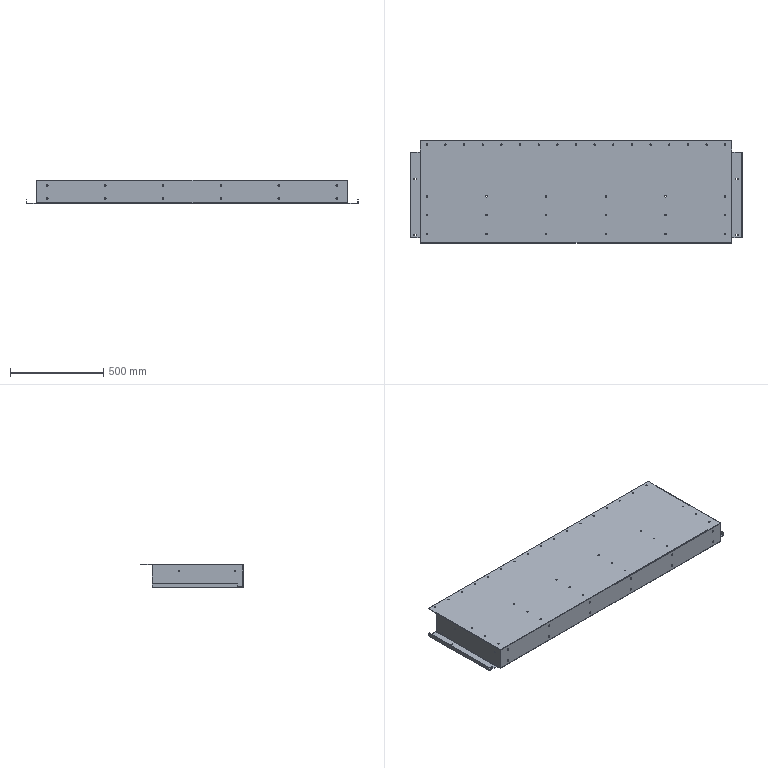Part | STEP file | TS-005-01 | 1 solid | 242 faces | box 1780 x 548 x 125 mm | volume 2679291 mm3 | cylinder 146 | plane 94 | spline 2 | commonest cylinder face diameters 8 x48 7 x34 5.4 x24 10.5 x24 0.4 x8 4.4 x8